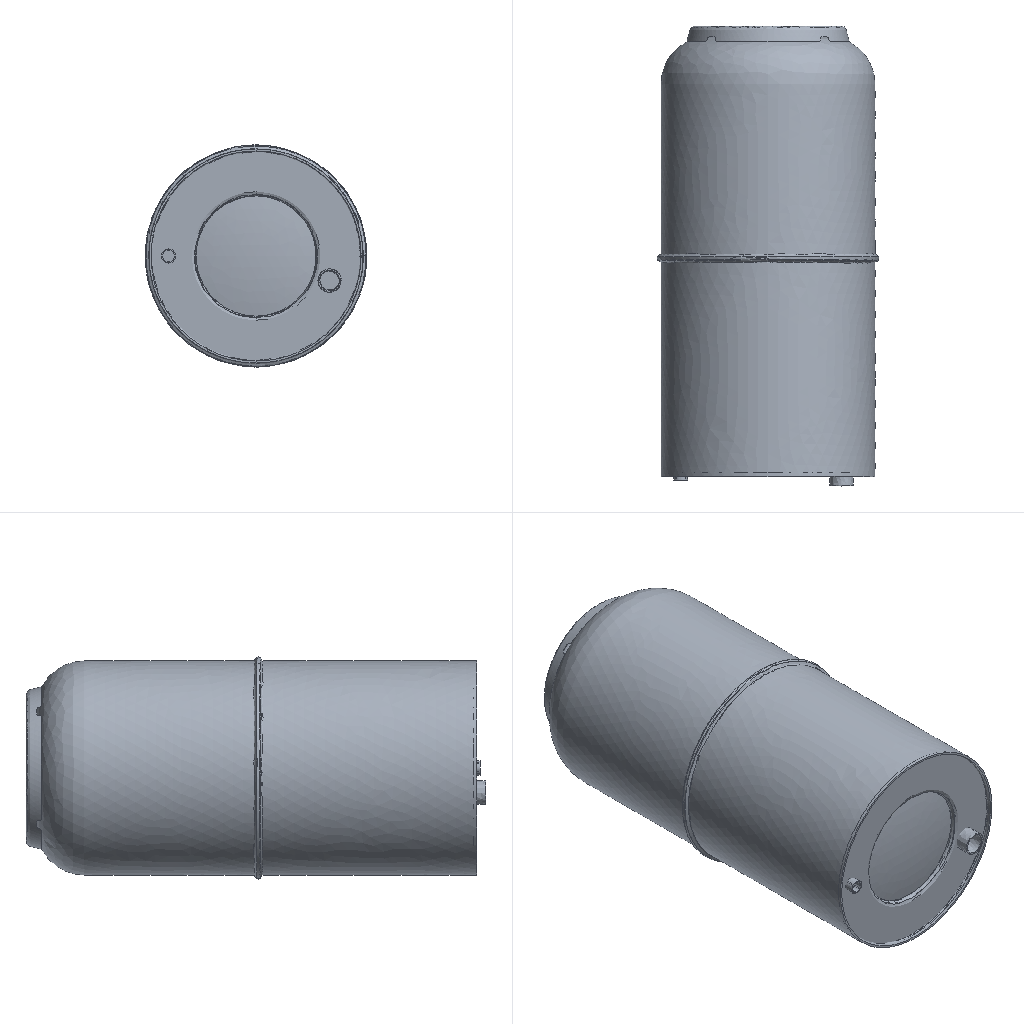Simulation study | ansys workbench
Ansys APDL input file, long lists of numbers shortened:
/batch
/config,noeldb,1     ! force off writing results to database
*get,_wallstrt,active,,time,wall
! ANSYS input file written by Workbench version 2024 R2
! File used for geometry attach:
/title,wbnew--___ (A5)
! ****** Begin Custom Load Command Snippet ******
/COM, ACT Extensions:
/COM,     LSDYNA, 2024.2
/COM,/COM,     ANSYSMotion, 2024.2
/COM,
! ****** End   Custom Load Command Snippet ******
*DIM,_wb_ProjectScratch_dir,string,248
_wb_ProjectScratch_dir(1) = ''
*DIM,_wb_SolverFiles_dir,string,248
_wb_SolverFiles_dir(1) = ''
*DIM,_wb_userfiles_dir,string,248
_wb_userfiles_dir(1) = ''
/com,--- Data in consistent NMM units. See Solving Units in the help system for more information.
/units,MPA
/nopr
/wb,file,start              !  signify a WB generated input file
/prep7
! Turn off shape checking because checks already performed inside WB mesher.
! See help system for more information.
SHPP,OFF,,NOWARN
/nolist
etcon,set             ! allow ANSYS to choose best KEYOP's for 180x elements, resets any applicable keyopt to MAPDL defaults
/com,*********** Nodes for the whole assembly ***********
nblock,3,,111691
(1i9,3e20.9e3)
   100406    -7.525578160E+01    -3.190000000E+02    -5.380866318E+00
! (101537 more lines like these left out)
-1
/wb,elem,start            !  set before creation of elements
/com,*********** Elements for Body 1 'Z_ASM_35_ASM|PRT0001_21|PRT0001_21' ***********
et,1,291
eblock,19,solid,,41186
(19i9)
        1        1        1        1        0        0        0        0       10        0        1     1222     3979     1223     4152    24811    24824    24807    24813
! (82371 more lines like these left out)
-1
/com,*********** Elements for Body 2 'Z_ASM_35_ASM|20X14_1|20X14_1' ***********
et,2,291
eblock,19,solid,,1068
(19i9)
        2        2        2        2        0        0        0        0       10        0    41187    81453    81537    81589    81690    82196    82698    82198    82203
! (2135 more lines like these left out)
-1
/com,*********** Elements for Body 3 'Z_ASM_35_ASM|DN15-1_1|DN15-1_1' ***********
et,3,291
eblock,19,solid,,2313
(19i9)
        3        3        3        3        0        0        0        0       10        0    42255    84534    84608    84567    84568    88980    89086    88973    88974
! (4625 more lines like these left out)
-1
/com,*********** Elements for Body 4 'Z_ASM_35_ASM|5_22|5_22' ***********
et,4,291
eblock,19,solid,,5247
(19i9)
        4        4        4        4        0        0        0        0       10        0    44568    89485    90565    90603    90604    92828    99020    92829    92830
! (10493 more lines like these left out)
-1
/com,*********** Elements for Body 5 'Z_ASM_35_ASM|DN6_35_2|DN6_35_2' ***********
et,5,279
eblock,19,solid,,156
(19i9)
        5        5        5        5        0        0        0        0       20        0    49815   100606   100658   100657   100607   100623   100672   100671   100624
! (311 more lines like these left out)
-1
/wb,elem,end               !  done creating elements
/com,*********** Send User Defined Coordinate System(s) ***********
csys,0
toffst,273.15,      ! Temperature offset from absolute zero
/wb,mat,start              !  starting to send materials
/com,*********** Send Materials ***********
Temperature = 'TEMP' ! Temperature
MP,DENS,1,7.75e-09,	! tonne mm^-3
MP,ALPX,1,1.7e-05,	! C^-1
MP,C,1,480000000,	! mm^2 s^-2 C^-1
MP,KXX,1,15.1,	! tonne mm s^-3 C^-1
MP,RSVX,1,0.00077,	! ohm mm
MP,EX,1,193000,	! tonne s^-2 mm^-1
MP,NUXY,1,0.31,
MP,MURX,1,1,
Temperature = 'TEMP' ! Temperature
MP,DENS,2,7.75e-09,	! tonne mm^-3
MP,ALPX,2,1.7e-05,	! C^-1
MP,C,2,480000000,	! mm^2 s^-2 C^-1
MP,KXX,2,15.1,	! tonne mm s^-3 C^-1
MP,RSVX,2,0.00077,	! ohm mm
MP,EX,2,193000,	! tonne s^-2 mm^-1
MP,NUXY,2,0.31,
MP,MURX,2,1,
Temperature = 'TEMP' ! Temperature
MP,DENS,3,7.75e-09,	! tonne mm^-3
MP,ALPX,3,1.7e-05,	! C^-1
MP,C,3,480000000,	! mm^2 s^-2 C^-1
MP,KXX,3,15.1,	! tonne mm s^-3 C^-1
MP,RSVX,3,0.00077,	! ohm mm
MP,EX,3,193000,	! tonne s^-2 mm^-1
MP,NUXY,3,0.31,
MP,MURX,3,1,
Temperature = 'TEMP' ! Temperature
MP,DENS,4,7.75e-09,	! tonne mm^-3
MP,ALPX,4,1.7e-05,	! C^-1
MP,C,4,480000000,	! mm^2 s^-2 C^-1
MP,KXX,4,15.1,	! tonne mm s^-3 C^-1
MP,RSVX,4,0.00077,	! ohm mm
MP,EX,4,193000,	! tonne s^-2 mm^-1
MP,NUXY,4,0.31,
MP,MURX,4,1,
Temperature = 'TEMP' ! Temperature
MP,DENS,5,7.75e-09,	! tonne mm^-3
MP,ALPX,5,1.7e-05,	! C^-1
MP,C,5,480000000,	! mm^2 s^-2 C^-1
MP,KXX,5,15.1,	! tonne mm s^-3 C^-1
MP,RSVX,5,0.00077,	! ohm mm
MP,EX,5,193000,	! tonne s^-2 mm^-1
MP,NUXY,5,0.31,
MP,MURX,5,1,
/wb,mat,end                !  done sending materials
!************************* Model Summary ********************
!Z_ASM_35_ASM|PRT0001_21|PRT0001_21,	304é¢,	matid,	1
!Z_ASM_35_ASM|20X14_1|20X14_1,	304é¢,	matid,	2
!Z_ASM_35_ASM|DN15-1_1|DN15-1_1,	304é¢,	matid,	3
!Z_ASM_35_ASM|5_22|5_22,	304é¢,	matid,	4
!Z_ASM_35_ASM|DN6_35_2|DN6_35_2,	304é¢,	matid,	5
!************************* End Model Summary ********************
! get the diagonal of the bounding box. Needed later for other things
*get,_xmin,node,,mnloc,x
*get,_ymin,node,,mnloc,y
*get,_zmin,node,,mnloc,z
*get,_xmax,node,,mxloc,x
*get,_ymax,node,,mxloc,y
*get,_zmax,node,,mxloc,z
_ASMDIAG=(_xmax-_xmin)*(_xmax-_xmin)+(_ymax-_ymin)*(_ymax-_ymin)+(_zmax-_zmin)*(_zmax-_zmin)
_ASMDIAG=SQRT(_ASMDIAG)
/wb,contact,start          !  starting to send contact
/com,*********** Create Contact "½Ó´¥ÇøÓò" ***********
/com,            Real Constant Set For Above Contact Is 7 & 6
*set,tid,7
*set,cid,6
r,tid
r,cid
et,tid,170
et,cid,174
eblock,10,,,49
(15i9)
    83777        7        7        7        0    12368    12346    12440    12440    79795    79798    12440    79960
! (48 more lines like these left out)
-1
eblock,10,,,49
(15i9)
    83826        6        6        6        0    12368    12346    12440    12440    79795    79798    12440    79960
! (48 more lines like these left out)
-1
eblock,10,,,56
(15i9)
    83875        6        7        6        0    81508    81520    81509    81509    82507    82512    81509    82506
! (55 more lines like these left out)
-1
eblock,10,,,56
(15i9)
    83931        7        6        7        0    81508    81520    81509    81509    82507    82512    81509    82506
! (55 more lines like these left out)
-1
keyo,cid,8,2               ! auto create asymmetric contact (from Program Controlled setting)
keyo,cid,10,0              ! adjust contact stiffness each NR iteration (from Program Controlled setting)
keyo,cid,12,5              ! bonded always
keyo,cid,18,1              ! small sliding turned on by application
keyo,cid,2,0               ! augmented Lagrange (from Program Controlled setting)
keyo,cid,4,0               ! on Gauss point (from Program Controlled setting)
keyo,cid,9,1               ! ignore initial gaps/penetration
keyo,cid,7,0               ! No Prediction
rmod,tid,3,10.      ! FKN
rmod,tid,5,0.       ! ICONT
rmod,tid,6,0.       ! PINB
rmod,tid,10,0.      ! CNOF
rmod,tid,12,0.      ! FKT
rmod,tid,36,39      ! WB DSID
rmod,cid,3,10.      ! FKN
rmod,cid,5,0.       ! ICONT
rmod,cid,6,0.       ! PINB
rmod,cid,10,0.      ! CNOF
rmod,cid,12,0.      ! FKT
rmod,cid,36,39      ! WB DSID
*set,_maxkxx,151000.
rmod,cid,14,_maxkxx/_ASMDIAG         ! TCC, Divide by Length since Traction Based
rmod,tid,14,_maxkxx/_ASMDIAG      ! TCC, Divide by Length since Traction Based
keyo,cid,1,2     ! Pure thermal contact
/com,*********** Create Contact "½Ó´¥ÇøÓò 2" ***********
/com,            Real Constant Set For Above Contact Is 9 & 8
*set,tid,9
*set,cid,8
r,tid
r,cid
et,tid,170
et,cid,174
eblock,10,,,17
(15i9)
    83987        9        9        9        0    12338    12368    12369    12369    79729    79959    12369    79730
! (16 more lines like these left out)
-1
eblock,10,,,17
(15i9)
    84004        8        8        8        0    12338    12368    12369    12369    79729    79959    12369    79730
! (16 more lines like these left out)
-1
eblock,10,,,28
(15i9)
    84021        8        9        8        0    83837    84450    84442    84442    86125    88506    84442    86123
! (27 more lines like these left out)
-1
eblock,10,,,28
(15i9)
    84049        9        8        9        0    83837    84450    84442    84442    86125    88506    84442    86123
! (27 more lines like these left out)
-1
keyo,cid,8,2               ! auto create asymmetric contact (from Program Controlled setting)
keyo,cid,10,0              ! adjust contact stiffness each NR iteration (from Program Controlled setting)
keyo,cid,12,5              ! bonded always
keyo,cid,18,1              ! small sliding turned on by application
keyo,cid,2,0               ! augmented Lagrange (from Program Controlled setting)
keyo,cid,4,0               ! on Gauss point (from Program Controlled setting)
keyo,cid,9,1               ! ignore initial gaps/penetration
keyo,cid,7,0               ! No Prediction
rmod,tid,3,10.      ! FKN
rmod,tid,5,0.       ! ICONT
rmod,tid,6,0.       ! PINB
rmod,tid,10,0.      ! CNOF
rmod,tid,12,0.      ! FKT
rmod,tid,36,42      ! WB DSID
rmod,cid,3,10.      ! FKN
rmod,cid,5,0.       ! ICONT
rmod,cid,6,0.       ! PINB
rmod,cid,10,0.      ! CNOF
rmod,cid,12,0.      ! FKT
rmod,cid,36,42      ! WB DSID
*set,_maxkxx,151000.
rmod,cid,14,_maxkxx/_ASMDIAG         ! TCC, Divide by Length since Traction Based
rmod,tid,14,_maxkxx/_ASMDIAG      ! TCC, Divide by Length since Traction Based
keyo,cid,1,2     ! Pure thermal contact
/com,*********** Create Contact "½Ó´¥ÇøÓò 3" ***********
/com,            Real Constant Set For Above Contact Is 11 & 10
*set,tid,11
*set,cid,10
r,tid
r,cid
et,tid,170
et,cid,174
eblock,10,,,130
(15i9)
    84077       11       11       11        0      199      198     4836     4836    15103    15106     4836    15111
! (129 more lines like these left out)
-1
eblock,10,,,130
(15i9)
    84207       10       10       10        0      199      198     4836     4836    15103    15106     4836    15111
! (129 more lines like these left out)
-1
eblock,10,,,144
(15i9)
    84337       10       11       10        0    89950    89949    89947    89947    96181    96173    89947    96174
! (143 more lines like these left out)
-1
eblock,10,,,144
(15i9)
    84481       11       10       11        0    89950    89949    89947    89947    96181    96173    89947    96174
! (143 more lines like these left out)
-1
keyo,cid,8,2               ! auto create asymmetric contact (from Program Controlled setting)
keyo,cid,10,0              ! adjust contact stiffness each NR iteration (from Program Controlled setting)
keyo,cid,12,5              ! bonded always
keyo,cid,18,1              ! small sliding turned on by application
keyo,cid,2,0               ! augmented Lagrange (from Program Controlled setting)
keyo,cid,4,0               ! on Gauss point (from Program Controlled setting)
keyo,cid,9,1               ! ignore initial gaps/penetration
keyo,cid,7,0               ! No Prediction
rmod,tid,3,10.      ! FKN
rmod,tid,5,0.       ! ICONT
rmod,tid,6,0.       ! PINB
rmod,tid,10,0.      ! CNOF
rmod,tid,12,0.      ! FKT
rmod,tid,36,45      ! WB DSID
rmod,cid,3,10.      ! FKN
rmod,cid,5,0.       ! ICONT
rmod,cid,6,0.       ! PINB
rmod,cid,10,0.      ! CNOF
rmod,cid,12,0.      ! FKT
rmod,cid,36,45      ! WB DSID
*set,_maxkxx,151000.
rmod,cid,14,_maxkxx/_ASMDIAG         ! TCC, Divide by Length since Traction Based
rmod,tid,14,_maxkxx/_ASMDIAG      ! TCC, Divide by Length since Traction Based
keyo,cid,1,2     ! Pure thermal contact
/com,*********** Create Contact "½Ó´¥ÇøÓò 4" ***********
/com,            Real Constant Set For Above Contact Is 13 & 12
*set,tid,13
*set,cid,12
r,tid
r,cid
et,tid,170
et,cid,174
eblock,10,,,28
(15i9)
    84625       13       13       13        0    12555      866    13117    13117    21080    21082    13117    80661
! (27 more lines like these left out)
-1
eblock,10,,,28
(15i9)
    84653       12       12       12        0    12555      866    13117    13117    21080    21082    13117    80661
! (27 more lines like these left out)
-1
eblock,10,,,39
(15i9)
    84681       12       13       12        0   100452   100445   100453   100453   100876   100877   100453   100894
! (38 more lines like these left out)
-1
eblock,10,,,39
(15i9)
    84720       13       12       13        0   100452   100445   100453   100453   100876   100877   100453   100894
! (38 more lines like these left out)
-1
keyo,cid,8,2               ! auto create asymmetric contact (from Program Controlled setting)
keyo,cid,10,0              ! adjust contact stiffness each NR iteration (from Program Controlled setting)
keyo,cid,12,5              ! bonded always
keyo,cid,18,1              ! small sliding turned on by application
keyo,cid,2,0               ! augmented Lagrange (from Program Controlled setting)
keyo,cid,4,0               ! on Gauss point (from Program Controlled setting)
keyo,cid,9,1               ! ignore initial gaps/penetration
keyo,cid,7,0               ! No Prediction
rmod,tid,3,10.      ! FKN
rmod,tid,5,0.       ! ICONT
rmod,tid,6,0.       ! PINB
rmod,tid,10,0.      ! CNOF
rmod,tid,12,0.      ! FKT
rmod,tid,36,48      ! WB DSID
rmod,cid,3,10.      ! FKN
rmod,cid,5,0.       ! ICONT
rmod,cid,6,0.       ! PINB
rmod,cid,10,0.      ! CNOF
rmod,cid,12,0.      ! FKT
rmod,cid,36,48      ! WB DSID
*set,_maxkxx,151000.
rmod,cid,14,_maxkxx/_ASMDIAG         ! TCC, Divide by Length since Traction Based
rmod,tid,14,_maxkxx/_ASMDIAG      ! TCC, Divide by Length since Traction Based
keyo,cid,1,2     ! Pure thermal contact
/com,*********** Create Contact "½Ó´¥ÇøÓò 5" ***********
/com,            Real Constant Set For Above Contact Is 15 & 14
*set,tid,15
*set,cid,14
r,tid
r,cid
et,tid,170
et,cid,174
eblock,10,,,74
(15i9)
    84759       15       15       15        0    81479    81495    81594    81594    82357    82451    81594    82364
! (73 more lines like these left out)
-1
eblock,10,,,74
(15i9)
    84833       14       14       14        0    81479    81495    81594    81594    82357    82451    81594    82364
! (73 more lines like these left out)
-1
eblock,10,,,73
(15i9)
    84907       14       15       14        0    83682    84442    84599    84599    85203    88507    84599    85205
! (72 more lines like these left out)
-1
eblock,10,,,73
(15i9)
    84980       15       14       15        0    83682    84442    84599    84599    85203    88507    84599    85205
! (72 more lines like these left out)
-1
keyo,cid,8,2               ! auto create asymmetric contact (from Program Controlled setting)
keyo,cid,10,0              ! adjust contact stiffness each NR iteration (from Program Controlled setting)
keyo,cid,12,5              ! bonded always
keyo,cid,18,1              ! small sliding turned on by application
keyo,cid,2,0               ! augmented Lagrange (from Program Controlled setting)
keyo,cid,4,0               ! on Gauss point (from Program Controlled setting)
keyo,cid,9,1               ! ignore initial gaps/penetration
keyo,cid,7,0               ! No Prediction
rmod,tid,3,10.      ! FKN
rmod,tid,5,0.       ! ICONT
rmod,tid,6,0.       ! PINB
rmod,tid,10,0.      ! CNOF
rmod,tid,12,0.      ! FKT
rmod,tid,36,51      ! WB DSID
rmod,cid,3,10.      ! FKN
rmod,cid,5,0.       ! ICONT
rmod,cid,6,0.       ! PINB
rmod,cid,10,0.      ! CNOF
rmod,cid,12,0.      ! FKT
rmod,cid,36,51      ! WB DSID
*set,_maxkxx,151000.
rmod,cid,14,_maxkxx/_ASMDIAG         ! TCC, Divide by Length since Traction Based
rmod,tid,14,_maxkxx/_ASMDIAG      ! TCC, Divide by Length since Traction Based
keyo,cid,1,2     ! Pure thermal contact
nsel,all
esel,all
/wb,contact,end            !  done creating contacts
/golist
/wb,load,start             !  starting to send loads
/com,*********** Define Temperature Constraint ***********
CMBLOCK,_CM65   ,NODE,    11826
(8i10)
      1112      1113      1114      1115      1116      1117      1118      1119
! (1478 more lines like these left out)
fcum,add                   ! add nodal forces up (needed in case have loads on the same edge,vertex)
fcum                       ! reset default on fcum command since done sending WB F loads
/com,*********** Create "______" ***********
et,16,152
eblock,10,,,9298
(15i9)
    85053       16       16       16        0      550      581     3000     3000    18492    18808     3000    18496
! (9297 more lines like these left out)
-1
esel,s,type,,16
keyop,16,8,2
keyop,16,13,0
esel,all
/com,*********** Create "ToAmbient" Radiation ***********
n,101539,_ASMDIAG*0.5*1,0.,0.
nsel,s,node,,101539
cm,_SPND82,node
nsel,all
et,17,152
keyop,17,5,1        !  Extra node
keyop,17,9,1        !  Use radiation with the form factor real constant
eblock,10,,,7257
(15i9)
    94351       17       17       17        0      251      252     4713     4713    15523    15532     4713    15526   101539
! (7256 more lines like these left out)
-1
esel,s,type,,17
mp,emis,17,0.86
r,17,1.,5.669e-011
stef,5.669e-011
esel,all
nsel,all
/com,***************** Define Uniform Initial temperature ***************
tunif,22.
/gst,on,on
fini
*get,_numnode,node,0,count
*get,_numelem,elem,0,count
*get, _MAXELEMNUM, elem, 0, NUM, MAX
*get, _MAXNODENUM, node, 0, NUM, MAX
*get, _MAXELEMTYPE, etyp, 0, NUM, MAX
*get, _MAXREALCONST, rcon, 0, NUM, MAX
/go
/wb,load,end               !  done creating loads
/com,--- Number of total nodes = %_numnode%
/com,--- Number of contact elements = 17831
/com,--- Number of spring elements = 0
/com,--- Number of bearing elements = 0
/com,--- Number of solid elements = 49970
/com,--- Number of condensed parts = 0
/com,--- Number of total elements = %_numelem%
*get,_wallbsol,active,,time,wall
/com,****************************************************************************
/com,*************************    SOLUTION       ********************************
/com,****************************************************************************
/solu
antype,0                   ! static analysis
!eqsl,sparse               ! using sparse solver which is default so no eqsl command needed
cntr,print,1               ! print out contact info and also make no initial contact an error
rescontrol,,none                 ! Do not keep any restart files
dmpoption,emat,no             ! Don't combine emat file for DANSYS
dmpoption,esav,no             ! Don't combine esav file for DANSYS
/com,****************************************************
/com,******************* SOLVE FOR LS 1 OF 20 ****************
d,_CM65,temp,96.
esel,s,type,,16
nsle
sf,all,conv,200000.,20.
nsel,all
esel,all
d,_SPND82,temp,22.
/nopr
/gopr
autots,on
nsub,1,10,1
time,4320.
outres,erase
outres,all,none
outres,nsol,all
outres,rsol,all
outres,eangl,all
outres,veng,all
outres,fflux,all,
outres,cont,all,
/nopr
esel,s,type,,16
esel,a,type,,17
cm,_elmisc,elem
esel,all
/gopr
outres,misc,all,_elmisc
cnvtol,heat,,1.e-003,,1.e-003 ! Program Controlled. Set MINREF equivalent of 1e-6 Watts
! *********** WB SOLVE COMMAND ***********
! check interactive state
*get,ANSINTER_,active,,int
*if,ANSINTER_,ne,0,then
/eof
*endif
solve
/com *************** Write FE CONNECTORS *********
CEWRITE,file,ce,,INTE
/com,****************************************************
/com,*************** FINISHED SOLVE FOR LS 1 *************
/com,****************************************************
/com,******************* SOLVE FOR LS 2 OF 20 ****************
/nopr
/gopr
autots,on
nsub,1,10,1
time,8640.
outres,erase
outres,all,none
outres,nsol,all
outres,rsol,all
outres,eangl,all
outres,veng,all
outres,fflux,all,
outres,cont,all,
outres,misc,all,_elmisc
cnvtol,heat,,1.e-003,,1.e-003 ! Program Controlled. Set MINREF equivalent of 1e-6 Watts
solve
/com,****************************************************
/com,*************** FINISHED SOLVE FOR LS 2 *************
/com,****************************************************
/com,******************* SOLVE FOR LS 3 OF 20 ****************
/nopr
/gopr
autots,on
nsub,1,10,1
time,12960.
outres,erase
outres,all,none
outres,nsol,all
outres,rsol,all
outres,eangl,all
outres,veng,all
outres,fflux,all,
outres,cont,all,
outres,misc,all,_elmisc
cnvtol,heat,,1.e-003,,1.e-003 ! Program Controlled. Set MINREF equivalent of 1e-6 Watts
solve
/com,****************************************************
/com,*************** FINISHED SOLVE FOR LS 3 *************
/com,****************************************************
/com,******************* SOLVE FOR LS 4 OF 20 ****************
/nopr
/gopr
autots,on
nsub,1,10,1
time,17280.
outres,erase
outres,all,none
outres,nsol,all
outres,rsol,all
outres,eangl,all
outres,veng,all
outres,fflux,all,
outres,cont,all,
outres,misc,all,_elmisc
cnvtol,heat,,1.e-003,,1.e-003 ! Program Controlled. Set MINREF equivalent of 1e-6 Watts
solve
/com,****************************************************
/com,*************** FINISHED SOLVE FOR LS 4 *************
/com,****************************************************
/com,******************* SOLVE FOR LS 5 OF 20 ****************
/nopr
/gopr
autots,on
nsub,1,10,1
time,21600.
outres,erase
outres,all,none
outres,nsol,all
outres,rsol,all
outres,eangl,all
outres,veng,all
outres,fflux,all,
outres,cont,all,
outres,misc,all,_elmisc
cnvtol,heat,,1.e-003,,1.e-003 ! Program Controlled. Set MINREF equivalent of 1e-6 Watts
solve
/com,****************************************************
/com,*************** FINISHED SOLVE FOR LS 5 *************
/com,****************************************************
/com,******************* SOLVE FOR LS 6 OF 20 ****************
/nopr
/gopr
autots,on
nsub,1,10,1
time,25920.
outres,erase
outres,all,none
outres,nsol,all
outres,rsol,all
outres,eangl,all
outres,veng,all
outres,fflux,all,
outres,cont,all,
outres,misc,all,_elmisc
cnvtol,heat,,1.e-003,,1.e-003 ! Program Controlled. Set MINREF equivalent of 1e-6 Watts
solve
/com,****************************************************
/com,*************** FINISHED SOLVE FOR LS 6 *************
/com,****************************************************
/com,******************* SOLVE FOR LS 7 OF 20 ****************
/nopr
/gopr
autots,on
nsub,1,10,1
time,30240.
outres,erase
outres,all,none
outres,nsol,all
outres,rsol,all
outres,eangl,all
outres,veng,all
outres,fflux,all,
outres,cont,all,
outres,misc,all,_elmisc
cnvtol,heat,,1.e-003,,1.e-003 ! Program Controlled. Set MINREF equivalent of 1e-6 Watts
solve
/com,****************************************************
/com,*************** FINISHED SOLVE FOR LS 7 *************
/com,****************************************************
/com,******************* SOLVE FOR LS 8 OF 20 ****************
/nopr
/gopr
autots,on
nsub,1,10,1
time,34560.
outres,erase
outres,all,none
outres,nsol,all
outres,rsol,all
outres,eangl,all
outres,veng,all
outres,fflux,all,
outres,cont,all,
outres,misc,all,_elmisc
cnvtol,heat,,1.e-003,,1.e-003 ! Program Controlled. Set MINREF equivalent of 1e-6 Watts
solve
/com,****************************************************
/com,*************** FINISHED SOLVE FOR LS 8 *************
/com,****************************************************
/com,******************* SOLVE FOR LS 9 OF 20 ****************
/nopr
/gopr
autots,on
nsub,1,10,1
time,38880.
outres,erase
outres,all,none
outres,nsol,all
outres,rsol,all
outres,eangl,all
outres,veng,all
outres,fflux,all,
outres,cont,all,
outres,misc,all,_elmisc
cnvtol,heat,,1.e-003,,1.e-003 ! Program Controlled. Set MINREF equivalent of 1e-6 Watts
solve
/com,****************************************************
/com,*************** FINISHED SOLVE FOR LS 9 *************
/com,****************************************************
/com,******************* SOLVE FOR LS 10 OF 20 ****************
/nopr
/gopr
autots,on
nsub,1,10,1
time,43200.
outres,erase
outres,all,none
outres,nsol,all
outres,rsol,all
outres,eangl,all
outres,veng,all
outres,fflux,all,
outres,cont,all,
outres,misc,all,_elmisc
cnvtol,heat,,1.e-003,,1.e-003 ! Program Controlled. Set MINREF equivalent of 1e-6 Watts
solve
/com,****************************************************
/com,*************** FINISHED SOLVE FOR LS 10 *************
/com,****************************************************
/com,******************* SOLVE FOR LS 11 OF 20 ****************
/nopr
/gopr
autots,on
nsub,1,10,1
time,47520.
outres,erase
outres,all,none
outres,nsol,all
outres,rsol,all
outres,eangl,all
outres,veng,all
outres,fflux,all,
outres,cont,all,
outres,misc,all,_elmisc
cnvtol,heat,,1.e-003,,1.e-003 ! Program Controlled. Set MINREF equivalent of 1e-6 Watts
solve
/com,****************************************************
/com,*************** FINISHED SOLVE FOR LS 11 *************
/com,****************************************************
/com,******************* SOLVE FOR LS 12 OF 20 ****************
/nopr
/gopr
autots,on
nsub,1,10,1
time,51840.
outres,erase
outres,all,none
outres,nsol,all
outres,rsol,all
outres,eangl,all
outres,veng,all
outres,fflux,all,
outres,cont,all,
outres,misc,all,_elmisc
cnvtol,heat,,1.e-003,,1.e-003 ! Program Controlled. Set MINREF equivalent of 1e-6 Watts
solve
/com,****************************************************
/com,*************** FINISHED SOLVE FOR LS 12 *************
/com,****************************************************
/com,******************* SOLVE FOR LS 13 OF 20 ****************
/nopr
/gopr
autots,on
nsub,1,10,1
time,56160.
outres,erase
outres,all,none
outres,nsol,all
outres,rsol,all
outres,eangl,all
outres,veng,all
outres,fflux,all,
outres,cont,all,
outres,misc,all,_elmisc
cnvtol,heat,,1.e-003,,1.e-003 ! Program Controlled. Set MINREF equivalent of 1e-6 Watts
solve
/com,****************************************************
/com,*************** FINISHED SOLVE FOR LS 13 *************
/com,****************************************************
/com,******************* SOLVE FOR LS 14 OF 20 ****************
/nopr
/gopr
autots,on
nsub,1,10,1
time,60480.
outres,erase
outres,all,none
outres,nsol,all
outres,rsol,all
outres,eangl,all
outres,veng,all
outres,fflux,all,
outres,cont,all,
outres,misc,all,_elmisc
cnvtol,heat,,1.e-003,,1.e-003 ! Program Controlled. Set MINREF equivalent of 1e-6 Watts
solve
/com,****************************************************
/com,*************** FINISHED SOLVE FOR LS 14 *************
/com,****************************************************
/com,******************* SOLVE FOR LS 15 OF 20 ****************
/nopr
/gopr
autots,on
nsub,1,10,1
time,64800.
outres,erase
outres,all,none
outres,nsol,all
outres,rsol,all
outres,eangl,all
outres,veng,all
outres,fflux,all,
outres,cont,all,
outres,misc,all,_elmisc
cnvtol,heat,,1.e-003,,1.e-003 ! Program Controlled. Set MINREF equivalent of 1e-6 Watts
solve
/com,****************************************************
/com,*************** FINISHED SOLVE FOR LS 15 *************
/com,****************************************************
/com,******************* SOLVE FOR LS 16 OF 20 ****************
/nopr
/gopr
autots,on
nsub,1,10,1
time,69120.
outres,erase
outres,all,none
outres,nsol,all
outres,rsol,all
outres,eangl,all
outres,veng,all
outres,fflux,all,
outres,cont,all,
outres,misc,all,_elmisc
cnvtol,heat,,1.e-003,,1.e-003 ! Program Controlled. Set MINREF equivalent of 1e-6 Watts
solve
/com,****************************************************
/com,*************** FINISHED SOLVE FOR LS 16 *************
/com,****************************************************
/com,******************* SOLVE FOR LS 17 OF 20 ****************
/nopr
/gopr
autots,on
nsub,1,10,1
time,73440.
outres,erase
outres,all,none
outres,nsol,all
outres,rsol,all
outres,eangl,all
outres,veng,all
outres,fflux,all,
outres,cont,all,
outres,misc,all,_elmisc
cnvtol,heat,,1.e-003,,1.e-003 ! Program Controlled. Set MINREF equivalent of 1e-6 Watts
solve
/com,****************************************************
/com,*************** FINISHED SOLVE FOR LS 17 *************
/com,****************************************************
/com,******************* SOLVE FOR LS 18 OF 20 ****************
/nopr
/gopr
autots,on
nsub,1,10,1
time,77760.
outres,erase
outres,all,none
outres,nsol,all
outres,rsol,all
outres,eangl,all
outres,veng,all
outres,fflux,all,
outres,cont,all,
outres,misc,all,_elmisc
cnvtol,heat,,1.e-003,,1.e-003 ! Program Controlled. Set MINREF equivalent of 1e-6 Watts
solve
/com,****************************************************
/com,*************** FINISHED SOLVE FOR LS 18 *************
/com,****************************************************
/com,******************* SOLVE FOR LS 19 OF 20 ****************
/nopr
/gopr
autots,on
nsub,1,10,1
time,82080.
outres,erase
outres,all,none
outres,nsol,all
outres,rsol,all
outres,eangl,all
outres,veng,all
outres,fflux,all,
outres,cont,all,
outres,misc,all,_elmisc
cnvtol,heat,,1.e-003,,1.e-003 ! Program Controlled. Set MINREF equivalent of 1e-6 Watts
solve
/com,****************************************************
/com,*************** FINISHED SOLVE FOR LS 19 *************
/com,****************************************************
/com,******************* SOLVE FOR LS 20 OF 20 ****************
/nopr
/gopr
autots,on
nsub,1,10,1
time,86400.
outres,erase
outres,all,none
outres,nsol,all
outres,rsol,all
outres,eangl,all
outres,veng,all
outres,fflux,all,
outres,cont,all,
outres,misc,all,_elmisc
cnvtol,heat,,1.e-003,,1.e-003 ! Program Controlled. Set MINREF equivalent of 1e-6 Watts
solve
/com,****************************************************
/com,*************** FINISHED SOLVE FOR LS 20 *************
*get,_wallasol,active,,time,wall
/post1
xmlo,ENCODING,ISO-8859-1
xmlo,parm
/xml,parm,xml
fini
/gopr
*get,_walldone,active,,time,wall
_preptime=(_wallbsol-_wallstrt)*3600
_solvtime=(_wallasol-_wallbsol)*3600
_posttime=(_walldone-_wallasol)*3600
_totaltim=(_walldone-_wallstrt)*3600
*get,_dlbratio,active,0,solu,dlbr
*get,_combtime,active,0,solu,comb
*get,_ssmode,active,0,solu,ssmm
*get,_ndofs,active,0,solu,ndof
/fclean				!clean distributed files
/com,--- Total number of nodes = %_numnode%
/com,--- Total number of elements = %_numelem%
/com,--- Element load balance ratio = %_dlbratio%
/com,--- Time to combine distributed files = %_combtime%
/com,--- Sparse memory mode = %_ssmode%
/com,--- Number of DOF = %_ndofs%
/wb,file,end               ! done with WB generated input